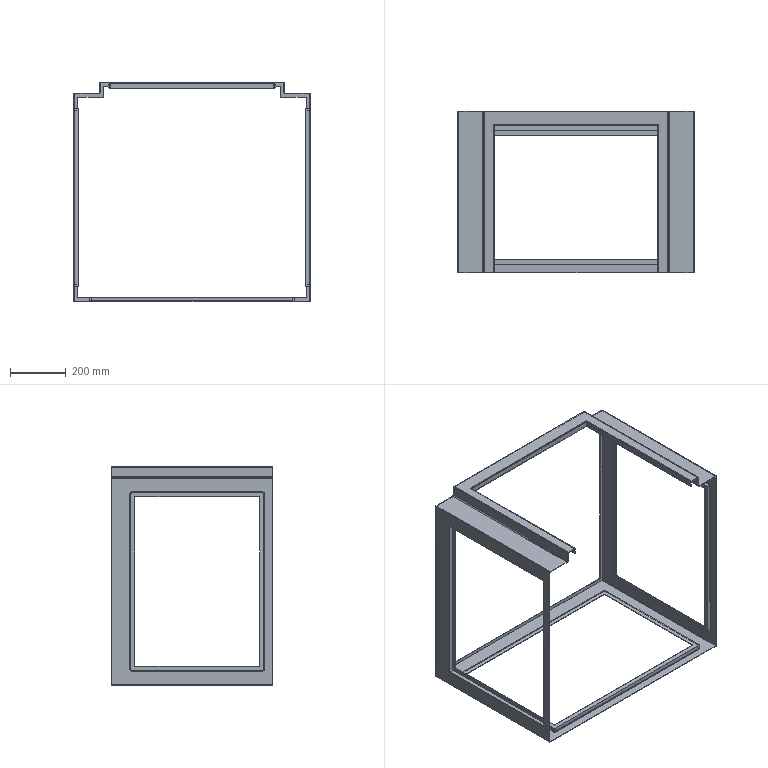Part | SolidWorks | features ICE 16, Fillet 6, HoleWzd 2, Extrusion 1, Shell 1 | 5 solids | 229 faces | box 851 x 582 x 791 mm | volume 1784461 mm3 | plane 140 | cylinder 77 | torus 12 | commonest cylinder face diameters 6 x39 4.2 x16 10 x14 2 x8